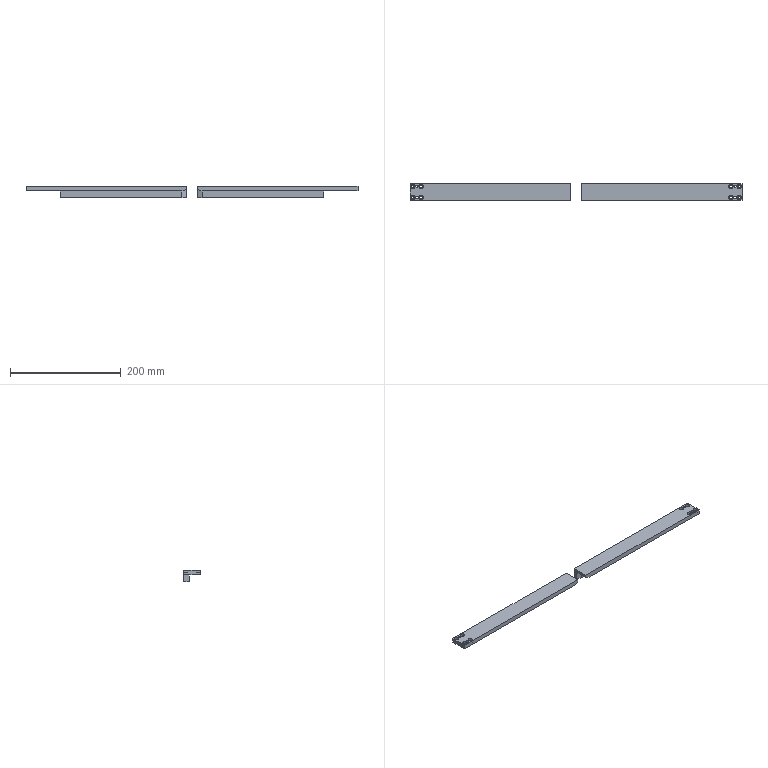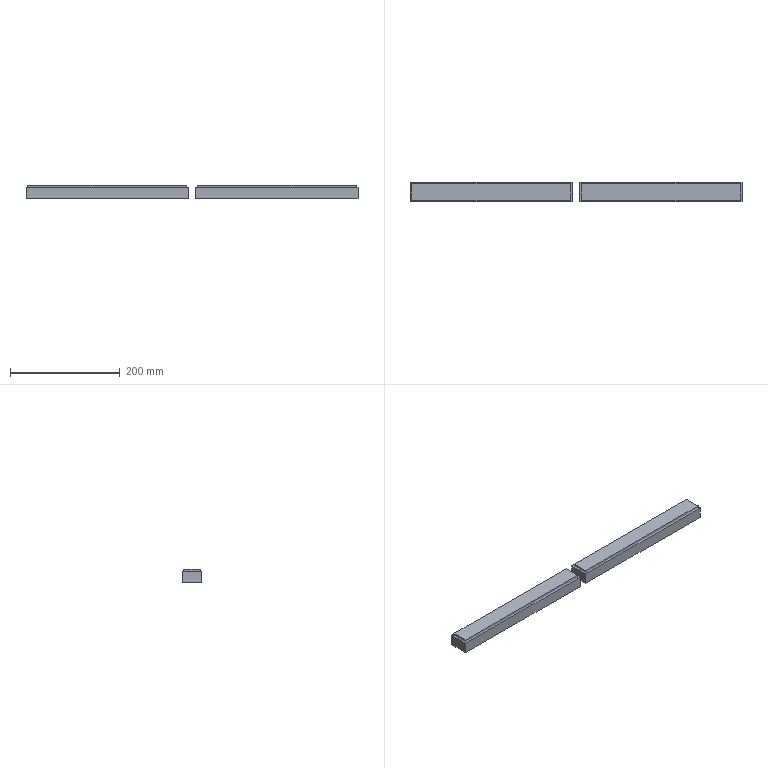CAM job | NX | 3-axis milling, drilling | part box 600 x 30 x 20 mm | stock box 606 x 36 x 25 mm
Tools:
number,name,description,diameter,corner_radius,flute_length,length,flutes
1,D50,Milling Tool-5 Parameters,50.0,0.0,50.0,75.0,2
2,D6A45,Milling Tool-5 Parameters,6.0,0.0,3.0,3.0,2
14,4.5ZT,Drilling Tool,4.5,0.0,35.0,50.0,2
12,2.5ZT,Drilling Tool,2.5,0.0,35.0,50.0,2
3,D10,Milling Tool-5 Parameters,10.0,0.0,50.0,75.0,2
4,D10JING,Milling Tool-5 Parameters,10.0,0.0,50.0,75.0,2
8,D6,Milling Tool-5 Parameters,6.0,0.0,50.0,75.0,2
20,D3,Milling Tool-5 Parameters,3.0,0.0,50.0,75.0,2
20,D6R0.5,Milling Tool-5 Parameters,6.0,0.5,50.0,75.0,2
Operations:
program,operation,operation_type,tool,method,geometry_group,spindle_rpm,surface_speed,feed_per_tooth,feed_cut,feed_plunge,cut_length_mm,path_length_mm,cut_time_min,machine_time_min
1-293-30-25_BLANK-VISE,FLOOR_WALL,VolumeBased25DMillingOperation,D50,METHOD,A,6500.0,1286.0,0.0962,1250.0,100.0,358.0,412.0,0.2864,0.2918
1-293-30-25_BLANK-VISE,DRILLING_COPY_1,Operation,D6A45,METHOD,A,3000.0,56.0,0.0333,200.0,0.0,27.6,182.766,0.138,0.1535
1-293-30-25_BLANK-VISE,DRILLING_COPY_1_COPY_COPY_1_COPY_1_COPY,Operation,4.5ZT,METHOD,A,2000.0,18.0,0.03,120.0,0.0,55.408,235.589,0.4617,0.4797
1-293-30-25_BLANK-VISE,DRILLING_COPY_1_COPY_COPY_1_COPY_1_COPY_COPY,Operation,2.5ZT,METHOD,A,2000.0,18.0,0.03,120.0,0.0,26.502,135.734,0.2209,0.2318
1-293-30-25_BLANK-VISE,ZLEVEL_PROFILE,ZLevelMilling,D10,METHOD,A,7000.0,219.0,0.2143,3000.0,1000.0,13547.609,13624.609,4.548,4.555
1-293-30-25_BLANK-VISE,ZLEVEL_PROFILE_COPY_COPY_1_COPY_COPY_COPY_1,ZLevelMilling,D10JING,METHOD,A,7000.0,219.0,0.0714,1000.0,100.0,674.548,774.548,0.6745,0.6845
1-293-30-25_BLANK-VISE,HOLE_MILLING_1,CylinderMilling,D6,METHOD,A,7000.0,131.0,0.1071,1500.0,100.0,284.779,590.379,0.1899,0.2204
1-293-30-25_BLANK-VISE,ZLEVEL_PROFILE_COPY_1_COPY,ZLevelMilling,D3,METHOD,A,7000.0,65.0,0.0929,1300.0,1000.0,263.194,415.602,0.2139,0.2291
1-293-30-25_BLANK-VISE,ZLEVEL_PROFILE_COPY_1_COPY_COPY_COPY_COPY_2_COPY,ZLevelMilling,D6A45,METHOD,A,7000.0,131.0,0.0714,1000.0,1000.0,765.617,1291.94,0.7656,0.8182
1-293-30-25_BLANK-VISE,COMPTOOL10_COPY,ZLevelMilling,D3,METHOD,A,7000.0,87.0,0.0607,850.0,1000.0,73.302,229.639,0.0859,0.1015
2-293-30-25_BLANK-VISE,FLOOR_WALL_COPY,VolumeBased25DMillingOperation,D50,METHOD,B,6500.0,1286.0,0.0962,1250.0,100.0,1760.0,3394.001,1.408,1.571
2-293-30-25_BLANK-VISE,FLOOR_WALL_1,VolumeBased25DMillingOperation,D10,METHOD,B,7000.0,219.0,0.2143,3000.0,1000.0,7415.401,7809.981,2.481,2.521
2-293-30-25_BLANK-VISE,FLOOR_WALL_1_COPY_1,VolumeBased25DMillingOperation,D10JING,METHOD,B,7000.0,87.0,0.0714,1000.0,100.0,2081.932,2494.618,2.082,2.124
2-293-30-25_BLANK-VISE,ZLEVEL_PROFILE_COPY_COPY_1_COPY_COPY_COPY_1_COPY_COPY,ZLevelMilling,D6R0.5,METHOD,B,7000.0,131.0,0.2143,3000.0,1000.0,1870.453,1957.668,0.6241,0.6328
2-293-30-25_BLANK-VISE,ZLEVEL_PROFILE_COPY_1_COPY_COPY_COPY_COPY_2_COPY_COPY,ZLevelMilling,D6A45,METHOD,B,7000.0,131.0,0.0714,1000.0,1000.0,483.635,545.635,0.4836,0.4898
2-293-30-25_BLANK-VISE,ZLEVEL_PROFILE_COPY_1_COPY_COPY_COPY_COPY_2_COPY_COPY_COPY,ZLevelMilling,D6A45,METHOD,B,7000.0,131.0,0.0714,1000.0,1000.0,440.122,1163.383,0.4401,0.5124
1SYM-293-30-25_BLANK-VISE,FLOOR_WALL_2,VolumeBased25DMillingOperation,D50,METHOD,A,6500.0,1286.0,0.0962,1250.0,100.0,358.0,412.0,0.2864,0.2918
1SYM-293-30-25_BLANK-VISE,DRILLING_COPY_1_1,Operation,D6A45,METHOD,A,3000.0,56.0,0.0333,200.0,0.0,27.6,182.766,0.138,0.1535
1SYM-293-30-25_BLANK-VISE,DRILLING_COPY_1_COPY_COPY_1_COPY_1_COPY_1,Operation,4.5ZT,METHOD,A,2000.0,18.0,0.03,120.0,0.0,55.408,235.589,0.4617,0.4797
1SYM-293-30-25_BLANK-VISE,DRILLING_COPY_1_COPY_COPY_1_COPY_1_COPY_COPY_1,Operation,2.5ZT,METHOD,A,2000.0,18.0,0.03,120.0,0.0,26.502,135.734,0.2209,0.2318
1SYM-293-30-25_BLANK-VISE,ZLEVEL_PROFILE_1,ZLevelMilling,D10,METHOD,A,7000.0,219.0,0.2143,3000.0,1000.0,13547.609,13624.609,4.548,4.555
1SYM-293-30-25_BLANK-VISE,ZLEVEL_PROFILE_COPY_COPY_1_COPY_COPY_COPY_1_1,ZLevelMilling,D10JING,METHOD,A,7000.0,219.0,0.0714,1000.0,100.0,674.548,774.548,0.6745,0.6845
1SYM-293-30-25_BLANK-VISE,HOLE_MILLING_1_1,CylinderMilling,D6,METHOD,A,7000.0,131.0,0.1071,1500.0,100.0,284.779,590.379,0.1899,0.2204
1SYM-293-30-25_BLANK-VISE,ZLEVEL_PROFILE_COPY_1_COPY_1,ZLevelMilling,D3,METHOD,A,7000.0,65.0,0.0929,1300.0,1000.0,263.411,415.819,0.2141,0.2293
1SYM-293-30-25_BLANK-VISE,ZLEVEL_PROFILE_COPY_1_COPY_COPY_COPY_COPY_2_COPY_1,ZLevelMilling,D6A45,METHOD,A,7000.0,131.0,0.0714,1000.0,1000.0,765.617,1559.483,0.7656,0.845
1SYM-293-30-25_BLANK-VISE,COMPTOOL10_COPY_1,ZLevelMilling,D3,METHOD,A,7000.0,87.0,0.0607,850.0,1000.0,73.343,229.111,0.0859,0.1015
2SYM-293-30-25_BLANK-VISE,FLOOR_WALL_COPY_1,VolumeBased25DMillingOperation,D50,METHOD,B,6500.0,1286.0,0.0962,1250.0,100.0,1760.0,3394.001,1.408,1.571
2SYM-293-30-25_BLANK-VISE,FLOOR_WALL_1_1,VolumeBased25DMillingOperation,D10,METHOD,B,7000.0,219.0,0.2143,3000.0,1000.0,7440.651,8281.532,2.5,2.584
2SYM-293-30-25_BLANK-VISE,FLOOR_WALL_1_COPY_1_1,VolumeBased25DMillingOperation,D10JING,METHOD,B,7000.0,87.0,0.0714,1000.0,100.0,2299.856,2454.186,2.3,2.32
2SYM-293-30-25_BLANK-VISE,ZLEVEL_PROFILE_COPY_COPY_1_COPY_COPY_COPY_1_COPY_COPY_1,ZLevelMilling,D6R0.5,METHOD,B,7000.0,131.0,0.2143,3000.0,1000.0,1870.453,1957.668,0.6241,0.6328
2SYM-293-30-25_BLANK-VISE,ZLEVEL_PROFILE_COPY_1_COPY_COPY_COPY_COPY_2_COPY_COPY_1,ZLevelMilling,D6A45,METHOD,B,7000.0,131.0,0.0714,1000.0,1000.0,483.647,545.647,0.4836,0.4898
2SYM-293-30-25_BLANK-VISE,ZLEVEL_PROFILE_COPY_1_COPY_COPY_COPY_COPY_2_COPY_COPY_COPY_1,ZLevelMilling,D6A45,METHOD,B,7000.0,131.0,0.0714,1000.0,1000.0,440.122,1389.778,0.4401,0.5351